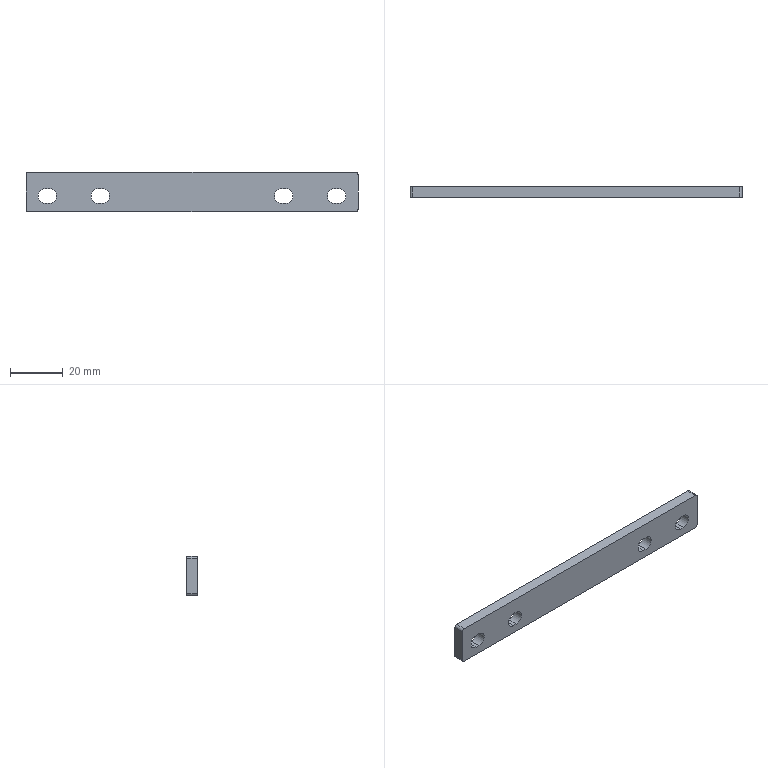Part | NX | features BREP 1 | 1 solid | 26 faces | box 125.75 x 4 x 15 mm | volume 7029 mm3 | plane 14 | cylinder 12 | commonest cylinder face diameters 5.5 x8 2 x4
STEP:
#1=CARTESIAN_POINT('',(147.026,-209.294,1985.218));
#2=VERTEX_POINT('',#1);
#3=CARTESIAN_POINT('',(147.026,-209.294,1998.218));
#4=VERTEX_POINT('',#3);
#5=CARTESIAN_POINT('',(147.026,-209.294,73.4));
#6=DIRECTION('',(0.,0.,1.));
#7=VECTOR('',#6,1000.);
#8=LINE('',#5,#7);
#9=EDGE_CURVE('',#2,#4,#8,.T.);
#10=ORIENTED_EDGE('',*,*,#9,.T.);
#11=CARTESIAN_POINT('',(146.026,-209.294,1999.218));
#12=VERTEX_POINT('',#11);
#13=CARTESIAN_POINT('',(146.026,-209.294,1998.218));
#14=DIRECTION('',(0.,1.,0.));
#15=DIRECTION('',(0.,0.,-1.));
#16=AXIS2_PLACEMENT_3D('',#13,#14,#15);
#17=CIRCLE('',#16,1.);
#18=EDGE_CURVE('',#12,#4,#17,.T.);
#19=ORIENTED_EDGE('',*,*,#18,.F.);
#20=CARTESIAN_POINT('',(22.276,-209.294,1999.218));
#21=VERTEX_POINT('',#20);
#22=CARTESIAN_POINT('',(1.713,-209.294,1999.218));
#23=DIRECTION('',(-1.,0.,0.));
#24=VECTOR('',#23,1000.);
#25=LINE('',#22,#24);
#26=EDGE_CURVE('',#12,#21,#25,.T.);
#27=ORIENTED_EDGE('',*,*,#26,.T.);
#28=CARTESIAN_POINT('',(21.276,-209.294,1998.218));
#29=VERTEX_POINT('',#28);
#30=CARTESIAN_POINT('',(22.276,-209.294,1998.218));
#31=DIRECTION('',(0.,1.,0.));
#32=DIRECTION('',(0.,0.,-1.));
#33=AXIS2_PLACEMENT_3D('',#30,#31,#32);
#34=CIRCLE('',#33,1.);
#35=EDGE_CURVE('',#29,#21,#34,.T.);
#36=ORIENTED_EDGE('',*,*,#35,.F.);
#37=CARTESIAN_POINT('',(21.276,-209.294,1985.218));
#38=VERTEX_POINT('',#37);
#39=CARTESIAN_POINT('',(21.276,-209.294,73.4));
#40=DIRECTION('',(0.,0.,-1.));
#41=VECTOR('',#40,1000.);
#42=LINE('',#39,#41);
#43=EDGE_CURVE('',#29,#38,#42,.T.);
#44=ORIENTED_EDGE('',*,*,#43,.T.);
#45=CARTESIAN_POINT('',(22.276,-209.294,1984.218));
#46=VERTEX_POINT('',#45);
#47=CARTESIAN_POINT('',(22.276,-209.294,1985.218));
#48=DIRECTION('',(0.,1.,0.));
#49=DIRECTION('',(0.,0.,1.));
#50=AXIS2_PLACEMENT_3D('',#47,#48,#49);
#51=CIRCLE('',#50,1.);
#52=EDGE_CURVE('',#46,#38,#51,.T.);
#53=ORIENTED_EDGE('',*,*,#52,.F.);
#54=CARTESIAN_POINT('',(146.026,-209.294,1984.218));
#55=VERTEX_POINT('',#54);
#56=CARTESIAN_POINT('',(1.713,-209.294,1984.218));
#57=DIRECTION('',(1.,0.,0.));
#58=VECTOR('',#57,1000.);
#59=LINE('',#56,#58);
#60=EDGE_CURVE('',#46,#55,#59,.T.);
#61=ORIENTED_EDGE('',*,*,#60,.T.);
#62=CARTESIAN_POINT('',(146.026,-209.294,1985.218));
#63=DIRECTION('',(0.,1.,0.));
#64=DIRECTION('',(0.,0.,-1.));
#65=AXIS2_PLACEMENT_3D('',#62,#63,#64);
#66=CIRCLE('',#65,1.);
#67=EDGE_CURVE('',#2,#55,#66,.T.);
#68=ORIENTED_EDGE('',*,*,#67,.F.);
#69=EDGE_LOOP('',(#10,#19,#27,#36,#44,#53,#61,#68));
#70=FACE_BOUND('',#69,.T.);
#71=CARTESIAN_POINT('',(139.651,-209.294,1992.95));
#72=VERTEX_POINT('',#71);
#73=CARTESIAN_POINT('',(139.651,-209.294,1987.45));
#74=VERTEX_POINT('',#73);
#75=CARTESIAN_POINT('',(139.651,-209.294,1990.2));
#76=DIRECTION('',(0.,1.,0.));
#77=DIRECTION('',(0.,0.,1.));
#78=AXIS2_PLACEMENT_3D('',#75,#76,#77);
#79=CIRCLE('',#78,2.75);
#80=EDGE_CURVE('',#72,#74,#79,.T.);
#81=ORIENTED_EDGE('',*,*,#80,.T.);
#82=CARTESIAN_POINT('',(138.151,-209.294,1987.45));
#83=VERTEX_POINT('',#82);
#84=CARTESIAN_POINT('',(48.651,-209.294,1987.45));
#85=DIRECTION('',(-1.,0.,0.));
#86=VECTOR('',#85,1000.);
#87=LINE('',#84,#86);
#88=EDGE_CURVE('',#74,#83,#87,.T.);
#89=ORIENTED_EDGE('',*,*,#88,.T.);
#90=CARTESIAN_POINT('',(138.151,-209.294,1992.95));
#91=VERTEX_POINT('',#90);
#92=CARTESIAN_POINT('',(138.151,-209.294,1990.2));
#93=DIRECTION('',(0.,1.,0.));
#94=DIRECTION('',(0.,0.,1.));
#95=AXIS2_PLACEMENT_3D('',#92,#93,#94);
#96=CIRCLE('',#95,2.75);
#97=EDGE_CURVE('',#83,#91,#96,.T.);
#98=ORIENTED_EDGE('',*,*,#97,.T.);
#99=CARTESIAN_POINT('',(50.151,-209.294,1992.95));
#100=DIRECTION('',(1.,0.,0.));
#101=VECTOR('',#100,1000.);
#102=LINE('',#99,#101);
#103=EDGE_CURVE('',#91,#72,#102,.T.);
#104=ORIENTED_EDGE('',*,*,#103,.T.);
#105=EDGE_LOOP('',(#81,#89,#98,#104));
#106=FACE_BOUND('',#105,.T.);
#107=CARTESIAN_POINT('',(118.151,-209.294,1992.95));
#108=VERTEX_POINT('',#107);
#109=CARTESIAN_POINT('',(119.651,-209.294,1992.95));
#110=VERTEX_POINT('',#109);
#111=CARTESIAN_POINT('',(50.151,-209.294,1992.95));
#112=DIRECTION('',(1.,0.,0.));
#113=VECTOR('',#112,1000.);
#114=LINE('',#111,#113);
#115=EDGE_CURVE('',#108,#110,#114,.T.);
#116=ORIENTED_EDGE('',*,*,#115,.T.);
#117=CARTESIAN_POINT('',(119.651,-209.294,1987.45));
#118=VERTEX_POINT('',#117);
#119=CARTESIAN_POINT('',(119.651,-209.294,1990.2));
#120=DIRECTION('',(0.,1.,0.));
#121=DIRECTION('',(0.,0.,1.));
#122=AXIS2_PLACEMENT_3D('',#119,#120,#121);
#123=CIRCLE('',#122,2.75);
#124=EDGE_CURVE('',#110,#118,#123,.T.);
#125=ORIENTED_EDGE('',*,*,#124,.T.);
#126=CARTESIAN_POINT('',(118.151,-209.294,1987.45));
#127=VERTEX_POINT('',#126);
#128=CARTESIAN_POINT('',(48.651,-209.294,1987.45));
#129=DIRECTION('',(-1.,0.,0.));
#130=VECTOR('',#129,1000.);
#131=LINE('',#128,#130);
#132=EDGE_CURVE('',#118,#127,#131,.T.);
#133=ORIENTED_EDGE('',*,*,#132,.T.);
#134=CARTESIAN_POINT('',(118.151,-209.294,1990.2));
#135=DIRECTION('',(0.,1.,0.));
#136=DIRECTION('',(0.,0.,1.));
#137=AXIS2_PLACEMENT_3D('',#134,#135,#136);
#138=CIRCLE('',#137,2.75);
#139=EDGE_CURVE('',#127,#108,#138,.T.);
#140=ORIENTED_EDGE('',*,*,#139,.T.);
#141=EDGE_LOOP('',(#116,#125,#133,#140));
#142=FACE_BOUND('',#141,.T.);
#143=CARTESIAN_POINT('',(30.151,-209.294,1992.95));
#144=VERTEX_POINT('',#143);
#145=CARTESIAN_POINT('',(30.151,-209.294,1987.45));
#146=VERTEX_POINT('',#145);
#147=CARTESIAN_POINT('',(30.151,-209.294,1990.2));
#148=DIRECTION('',(0.,1.,0.));
#149=DIRECTION('',(0.,0.,-1.));
#150=AXIS2_PLACEMENT_3D('',#147,#148,#149);
#151=CIRCLE('',#150,2.75);
#152=EDGE_CURVE('',#144,#146,#151,.T.);
#153=ORIENTED_EDGE('',*,*,#152,.T.);
#154=CARTESIAN_POINT('',(28.651,-209.294,1987.45));
#155=VERTEX_POINT('',#154);
#156=CARTESIAN_POINT('',(48.651,-209.294,1987.45));
#157=DIRECTION('',(-1.,0.,0.));
#158=VECTOR('',#157,1000.);
#159=LINE('',#156,#158);
#160=EDGE_CURVE('',#146,#155,#159,.T.);
#161=ORIENTED_EDGE('',*,*,#160,.T.);
#162=CARTESIAN_POINT('',(28.651,-209.294,1992.95));
#163=VERTEX_POINT('',#162);
#164=CARTESIAN_POINT('',(28.651,-209.294,1990.2));
#165=DIRECTION('',(0.,1.,0.));
#166=DIRECTION('',(0.,0.,-1.));
#167=AXIS2_PLACEMENT_3D('',#164,#165,#166);
#168=CIRCLE('',#167,2.75);
#169=EDGE_CURVE('',#155,#163,#168,.T.);
#170=ORIENTED_EDGE('',*,*,#169,.T.);
#171=CARTESIAN_POINT('',(50.151,-209.294,1992.95));
#172=DIRECTION('',(1.,0.,0.));
#173=VECTOR('',#172,1000.);
#174=LINE('',#171,#173);
#175=EDGE_CURVE('',#163,#144,#174,.T.);
#176=ORIENTED_EDGE('',*,*,#175,.T.);
#177=EDGE_LOOP('',(#153,#161,#170,#176));
#178=FACE_BOUND('',#177,.T.);
#179=CARTESIAN_POINT('',(50.151,-209.294,1992.95));
#180=VERTEX_POINT('',#179);
#181=CARTESIAN_POINT('',(50.151,-209.294,1987.45));
#182=VERTEX_POINT('',#181);
#183=CARTESIAN_POINT('',(50.151,-209.294,1990.2));
#184=DIRECTION('',(0.,1.,0.));
#185=DIRECTION('',(0.,0.,-1.));
#186=AXIS2_PLACEMENT_3D('',#183,#184,#185);
#187=CIRCLE('',#186,2.75);
#188=EDGE_CURVE('',#180,#182,#187,.T.);
#189=ORIENTED_EDGE('',*,*,#188,.T.);
#190=CARTESIAN_POINT('',(48.651,-209.294,1987.45));
#191=VERTEX_POINT('',#190);
#192=CARTESIAN_POINT('',(48.651,-209.294,1987.45));
#193=DIRECTION('',(-1.,0.,0.));
#194=VECTOR('',#193,1000.);
#195=LINE('',#192,#194);
#196=EDGE_CURVE('',#182,#191,#195,.T.);
#197=ORIENTED_EDGE('',*,*,#196,.T.);
#198=CARTESIAN_POINT('',(48.651,-209.294,1992.95));
#199=VERTEX_POINT('',#198);
#200=CARTESIAN_POINT('',(48.651,-209.294,1990.2));
#201=DIRECTION('',(0.,1.,0.));
#202=DIRECTION('',(0.,0.,-1.));
#203=AXIS2_PLACEMENT_3D('',#200,#201,#202);
#204=CIRCLE('',#203,2.75);
#205=EDGE_CURVE('',#191,#199,#204,.T.);
#206=ORIENTED_EDGE('',*,*,#205,.T.);
#207=CARTESIAN_POINT('',(50.151,-209.294,1992.95));
#208=DIRECTION('',(1.,0.,0.));
#209=VECTOR('',#208,1000.);
#210=LINE('',#207,#209);
#211=EDGE_CURVE('',#199,#180,#210,.T.);
#212=ORIENTED_EDGE('',*,*,#211,.T.);
#213=EDGE_LOOP('',(#189,#197,#206,#212));
#214=FACE_BOUND('',#213,.T.);
#215=CARTESIAN_POINT('',(1.713,-209.294,73.4));
#216=DIRECTION('',(0.,-1.,0.));
#217=DIRECTION('',(0.,0.,1.));
#218=AXIS2_PLACEMENT_3D('',#215,#216,#217);
#219=PLANE('',#218);
#220=ADVANCED_FACE('',(#70,#106,#142,#178,#214),#219,.T.);
#221=CARTESIAN_POINT('',(147.026,-205.294,1985.218));
#222=VERTEX_POINT('',#221);
#223=CARTESIAN_POINT('',(147.026,-206.294,1985.218));
#224=DIRECTION('',(0.,-1.,0.));
#225=VECTOR('',#224,1000.);
#226=LINE('',#223,#225);
#227=EDGE_CURVE('',#222,#2,#226,.T.);
#228=ORIENTED_EDGE('',*,*,#227,.F.);
#229=CARTESIAN_POINT('',(147.026,-205.294,1998.218));
#230=VERTEX_POINT('',#229);
#231=CARTESIAN_POINT('',(147.026,-205.294,2020.218));
#232=DIRECTION('',(0.,0.,-1.));
#233=VECTOR('',#232,1000.);
#234=LINE('',#231,#233);
#235=EDGE_CURVE('',#230,#222,#234,.T.);
#236=ORIENTED_EDGE('',*,*,#235,.F.);
#237=CARTESIAN_POINT('',(147.026,-206.294,1998.218));
#238=DIRECTION('',(0.,1.,0.));
#239=VECTOR('',#238,1000.);
#240=LINE('',#237,#239);
#241=EDGE_CURVE('',#4,#230,#240,.T.);
#242=ORIENTED_EDGE('',*,*,#241,.F.);
#243=ORIENTED_EDGE('',*,*,#9,.F.);
#244=EDGE_LOOP('',(#228,#236,#242,#243));
#245=FACE_BOUND('',#244,.T.);
#246=CARTESIAN_POINT('',(147.026,-206.294,2020.218));
#247=DIRECTION('',(-1.,0.,0.));
#248=DIRECTION('',(0.,0.,-1.));
#249=AXIS2_PLACEMENT_3D('',#246,#247,#248);
#250=PLANE('',#249);
#251=ADVANCED_FACE('',(#245),#250,.F.);
#252=CARTESIAN_POINT('',(22.276,-205.294,1984.218));
#253=VERTEX_POINT('',#252);
#254=CARTESIAN_POINT('',(22.276,-206.294,1984.218));
#255=DIRECTION('',(0.,1.,0.));
#256=VECTOR('',#255,1000.);
#257=LINE('',#254,#256);
#258=EDGE_CURVE('',#46,#253,#257,.T.);
#259=ORIENTED_EDGE('',*,*,#258,.T.);
#260=CARTESIAN_POINT('',(146.026,-205.294,1984.218));
#261=VERTEX_POINT('',#260);
#262=CARTESIAN_POINT('',(21.276,-205.294,1984.218));
#263=DIRECTION('',(1.,0.,0.));
#264=VECTOR('',#263,1000.);
#265=LINE('',#262,#264);
#266=EDGE_CURVE('',#253,#261,#265,.T.);
#267=ORIENTED_EDGE('',*,*,#266,.T.);
#268=CARTESIAN_POINT('',(146.026,-206.294,1984.218));
#269=DIRECTION('',(0.,-1.,0.));
#270=VECTOR('',#269,1000.);
#271=LINE('',#268,#270);
#272=EDGE_CURVE('',#261,#55,#271,.T.);
#273=ORIENTED_EDGE('',*,*,#272,.T.);
#274=ORIENTED_EDGE('',*,*,#60,.F.);
#275=EDGE_LOOP('',(#259,#267,#273,#274));
#276=FACE_BOUND('',#275,.T.);
#277=CARTESIAN_POINT('',(21.276,-206.294,1984.218));
#278=DIRECTION('',(0.,0.,-1.));
#279=DIRECTION('',(1.,0.,0.));
#280=AXIS2_PLACEMENT_3D('',#277,#278,#279);
#281=PLANE('',#280);
#282=ADVANCED_FACE('',(#276),#281,.T.);
#283=CARTESIAN_POINT('',(21.276,-205.294,1998.218));
#284=VERTEX_POINT('',#283);
#285=CARTESIAN_POINT('',(21.276,-205.294,1985.218));
#286=VERTEX_POINT('',#285);
#287=CARTESIAN_POINT('',(21.276,-205.294,2020.218));
#288=DIRECTION('',(0.,0.,-1.));
#289=VECTOR('',#288,1000.);
#290=LINE('',#287,#289);
#291=EDGE_CURVE('',#284,#286,#290,.T.);
#292=ORIENTED_EDGE('',*,*,#291,.T.);
#293=CARTESIAN_POINT('',(21.276,-206.294,1985.218));
#294=DIRECTION('',(0.,-1.,0.));
#295=VECTOR('',#294,1000.);
#296=LINE('',#293,#295);
#297=EDGE_CURVE('',#286,#38,#296,.T.);
#298=ORIENTED_EDGE('',*,*,#297,.T.);
#299=ORIENTED_EDGE('',*,*,#43,.F.);
#300=CARTESIAN_POINT('',(21.276,-206.294,1998.218));
#301=DIRECTION('',(0.,1.,0.));
#302=VECTOR('',#301,1000.);
#303=LINE('',#300,#302);
#304=EDGE_CURVE('',#29,#284,#303,.T.);
#305=ORIENTED_EDGE('',*,*,#304,.T.);
#306=EDGE_LOOP('',(#292,#298,#299,#305));
#307=FACE_BOUND('',#306,.T.);
#308=CARTESIAN_POINT('',(21.276,-206.294,2020.218));
#309=DIRECTION('',(-1.,0.,0.));
#310=DIRECTION('',(0.,0.,-1.));
#311=AXIS2_PLACEMENT_3D('',#308,#309,#310);
#312=PLANE('',#311);
#313=ADVANCED_FACE('',(#307),#312,.T.);
#314=ORIENTED_EDGE('',*,*,#26,.F.);
#315=CARTESIAN_POINT('',(146.026,-205.294,1999.218));
#316=VERTEX_POINT('',#315);
#317=CARTESIAN_POINT('',(146.026,-206.294,1999.218));
#318=DIRECTION('',(0.,1.,0.));
#319=VECTOR('',#318,1000.);
#320=LINE('',#317,#319);
#321=EDGE_CURVE('',#12,#316,#320,.T.);
#322=ORIENTED_EDGE('',*,*,#321,.T.);
#323=CARTESIAN_POINT('',(22.276,-205.294,1999.218));
#324=VERTEX_POINT('',#323);
#325=CARTESIAN_POINT('',(151.826,-205.294,1999.218));
#326=DIRECTION('',(-1.,0.,0.));
#327=VECTOR('',#326,1000.);
#328=LINE('',#325,#327);
#329=EDGE_CURVE('',#316,#324,#328,.T.);
#330=ORIENTED_EDGE('',*,*,#329,.T.);
#331=CARTESIAN_POINT('',(22.276,-206.294,1999.218));
#332=DIRECTION('',(0.,-1.,0.));
#333=VECTOR('',#332,1000.);
#334=LINE('',#331,#333);
#335=EDGE_CURVE('',#324,#21,#334,.T.);
#336=ORIENTED_EDGE('',*,*,#335,.T.);
#337=EDGE_LOOP('',(#314,#322,#330,#336));
#338=FACE_BOUND('',#337,.T.);
#339=CARTESIAN_POINT('',(151.826,-206.294,1999.218));
#340=DIRECTION('',(0.,0.,1.));
#341=DIRECTION('',(-1.,0.,0.));
#342=AXIS2_PLACEMENT_3D('',#339,#340,#341);
#343=PLANE('',#342);
#344=ADVANCED_FACE('',(#338),#343,.T.);
#345=ORIENTED_EDGE('',*,*,#80,.F.);
#346=CARTESIAN_POINT('',(139.651,-205.294,1992.95));
#347=VERTEX_POINT('',#346);
#348=CARTESIAN_POINT('',(139.651,-206.294,1992.95));
#349=DIRECTION('',(0.,-1.,0.));
#350=VECTOR('',#349,1000.);
#351=LINE('',#348,#350);
#352=EDGE_CURVE('',#347,#72,#351,.T.);
#353=ORIENTED_EDGE('',*,*,#352,.F.);
#354=CARTESIAN_POINT('',(139.651,-205.294,1987.45));
#355=VERTEX_POINT('',#354);
#356=CARTESIAN_POINT('',(139.651,-205.294,1990.2));
#357=DIRECTION('',(0.,-1.,0.));
#358=DIRECTION('',(0.,0.,1.));
#359=AXIS2_PLACEMENT_3D('',#356,#357,#358);
#360=CIRCLE('',#359,2.75);
#361=EDGE_CURVE('',#355,#347,#360,.T.);
#362=ORIENTED_EDGE('',*,*,#361,.F.);
#363=CARTESIAN_POINT('',(139.651,-206.294,1987.45));
#364=DIRECTION('',(0.,1.,0.));
#365=VECTOR('',#364,1000.);
#366=LINE('',#363,#365);
#367=EDGE_CURVE('',#74,#355,#366,.T.);
#368=ORIENTED_EDGE('',*,*,#367,.F.);
#369=EDGE_LOOP('',(#345,#353,#362,#368));
#370=FACE_BOUND('',#369,.T.);
#371=CARTESIAN_POINT('',(139.651,-206.294,1990.2));
#372=DIRECTION('',(0.,1.,0.));
#373=DIRECTION('',(0.,0.,-1.));
#374=AXIS2_PLACEMENT_3D('',#371,#372,#373);
#375=CYLINDRICAL_SURFACE('',#374,2.75);
#376=ADVANCED_FACE('',(#370),#375,.F.);
#377=ORIENTED_EDGE('',*,*,#97,.F.);
#378=CARTESIAN_POINT('',(138.151,-205.294,1987.45));
#379=VERTEX_POINT('',#378);
#380=CARTESIAN_POINT('',(138.151,-206.294,1987.45));
#381=DIRECTION('',(0.,-1.,0.));
#382=VECTOR('',#381,1000.);
#383=LINE('',#380,#382);
#384=EDGE_CURVE('',#379,#83,#383,.T.);
#385=ORIENTED_EDGE('',*,*,#384,.F.);
#386=CARTESIAN_POINT('',(138.151,-205.294,1992.95));
#387=VERTEX_POINT('',#386);
#388=CARTESIAN_POINT('',(138.151,-205.294,1990.2));
#389=DIRECTION('',(0.,-1.,0.));
#390=DIRECTION('',(0.,0.,1.));
#391=AXIS2_PLACEMENT_3D('',#388,#389,#390);
#392=CIRCLE('',#391,2.75);
#393=EDGE_CURVE('',#387,#379,#392,.T.);
#394=ORIENTED_EDGE('',*,*,#393,.F.);
#395=CARTESIAN_POINT('',(138.151,-206.294,1992.95));
#396=DIRECTION('',(0.,1.,0.));
#397=VECTOR('',#396,1000.);
#398=LINE('',#395,#397);
#399=EDGE_CURVE('',#91,#387,#398,.T.);
#400=ORIENTED_EDGE('',*,*,#399,.F.);
#401=EDGE_LOOP('',(#377,#385,#394,#400));
#402=FACE_BOUND('',#401,.T.);
#403=CARTESIAN_POINT('',(138.151,-206.294,1990.2));
#404=DIRECTION('',(0.,1.,0.));
#405=DIRECTION('',(0.,0.,-1.));
#406=AXIS2_PLACEMENT_3D('',#403,#404,#405);
#407=CYLINDRICAL_SURFACE('',#406,2.75);
#408=ADVANCED_FACE('',(#402),#407,.F.);
#409=ORIENTED_EDGE('',*,*,#124,.F.);
#410=CARTESIAN_POINT('',(119.651,-205.294,1992.95));
#411=VERTEX_POINT('',#410);
#412=CARTESIAN_POINT('',(119.651,-206.294,1992.95));
#413=DIRECTION('',(0.,-1.,0.));
#414=VECTOR('',#413,1000.);
#415=LINE('',#412,#414);
#416=EDGE_CURVE('',#411,#110,#415,.T.);
#417=ORIENTED_EDGE('',*,*,#416,.F.);
#418=CARTESIAN_POINT('',(119.651,-205.294,1987.45));
#419=VERTEX_POINT('',#418);
#420=CARTESIAN_POINT('',(119.651,-205.294,1990.2));
#421=DIRECTION('',(0.,-1.,0.));
#422=DIRECTION('',(0.,0.,1.));
#423=AXIS2_PLACEMENT_3D('',#420,#421,#422);
#424=CIRCLE('',#423,2.75);
#425=EDGE_CURVE('',#419,#411,#424,.T.);
#426=ORIENTED_EDGE('',*,*,#425,.F.);
#427=CARTESIAN_POINT('',(119.651,-206.294,1987.45));
#428=DIRECTION('',(0.,1.,0.));
#429=VECTOR('',#428,1000.);
#430=LINE('',#427,#429);
#431=EDGE_CURVE('',#118,#419,#430,.T.);
#432=ORIENTED_EDGE('',*,*,#431,.F.);
#433=EDGE_LOOP('',(#409,#417,#426,#432));
#434=FACE_BOUND('',#433,.T.);
#435=CARTESIAN_POINT('',(119.651,-206.294,1990.2));
#436=DIRECTION('',(0.,1.,0.));
#437=DIRECTION('',(0.,0.,-1.));
#438=AXIS2_PLACEMENT_3D('',#435,#436,#437);
#439=CYLINDRICAL_SURFACE('',#438,2.75);
#440=ADVANCED_FACE('',(#434),#439,.F.);
#441=CARTESIAN_POINT('',(118.151,-205.294,1992.95));
#442=VERTEX_POINT('',#441);
#443=CARTESIAN_POINT('',(118.151,-205.294,1987.45));
#444=VERTEX_POINT('',#443);
#445=CARTESIAN_POINT('',(118.151,-205.294,1990.2));
#446=DIRECTION('',(0.,-1.,0.));
#447=DIRECTION('',(0.,0.,1.));
#448=AXIS2_PLACEMENT_3D('',#445,#446,#447);
#449=CIRCLE('',#448,2.75);
#450=EDGE_CURVE('',#442,#444,#449,.T.);
#451=ORIENTED_EDGE('',*,*,#450,.F.);
#452=CARTESIAN_POINT('',(118.151,-206.294,1992.95));
#453=DIRECTION('',(0.,1.,0.));
#454=VECTOR('',#453,1000.);
#455=LINE('',#452,#454);
#456=EDGE_CURVE('',#108,#442,#455,.T.);
#457=ORIENTED_EDGE('',*,*,#456,.F.);
#458=ORIENTED_EDGE('',*,*,#139,.F.);
#459=CARTESIAN_POINT('',(118.151,-206.294,1987.45));
#460=DIRECTION('',(0.,-1.,0.));
#461=VECTOR('',#460,1000.);
#462=LINE('',#459,#461);
#463=EDGE_CURVE('',#444,#127,#462,.T.);
#464=ORIENTED_EDGE('',*,*,#463,.F.);
#465=EDGE_LOOP('',(#451,#457,#458,#464));
#466=FACE_BOUND('',#465,.T.);
#467=CARTESIAN_POINT('',(118.151,-206.294,1990.2));
#468=DIRECTION('',(0.,1.,0.));
#469=DIRECTION('',(0.,0.,-1.));
#470=AXIS2_PLACEMENT_3D('',#467,#468,#469);
#471=CYLINDRICAL_SURFACE('',#470,2.75);
#472=ADVANCED_FACE('',(#466),#471,.F.);
#473=ORIENTED_EDGE('',*,*,#152,.F.);
#474=CARTESIAN_POINT('',(30.151,-205.294,1992.95));
#475=VERTEX_POINT('',#474);
#476=CARTESIAN_POINT('',(30.151,-206.294,1992.95));
#477=DIRECTION('',(0.,-1.,0.));
#478=VECTOR('',#477,1000.);
#479=LINE('',#476,#478);
#480=EDGE_CURVE('',#475,#144,#479,.T.);
#481=ORIENTED_EDGE('',*,*,#480,.F.);
#482=CARTESIAN_POINT('',(30.151,-205.294,1987.45));
#483=VERTEX_POINT('',#482);
#484=CARTESIAN_POINT('',(30.151,-205.294,1990.2));
#485=DIRECTION('',(0.,-1.,0.));
#486=DIRECTION('',(0.,0.,-1.));
#487=AXIS2_PLACEMENT_3D('',#484,#485,#486);
#488=CIRCLE('',#487,2.75);
#489=EDGE_CURVE('',#483,#475,#488,.T.);
#490=ORIENTED_EDGE('',*,*,#489,.F.);
#491=CARTESIAN_POINT('',(30.151,-206.294,1987.45));
#492=DIRECTION('',(0.,1.,0.));
#493=VECTOR('',#492,1000.);
#494=LINE('',#491,#493);
#495=EDGE_CURVE('',#146,#483,#494,.T.);
#496=ORIENTED_EDGE('',*,*,#495,.F.);
#497=EDGE_LOOP('',(#473,#481,#490,#496));
#498=FACE_BOUND('',#497,.T.);
#499=CARTESIAN_POINT('',(30.151,-206.294,1990.2));
#500=DIRECTION('',(0.,-1.,0.));
#501=DIRECTION('',(0.,0.,1.));
#502=AXIS2_PLACEMENT_3D('',#499,#500,#501);
#503=CYLINDRICAL_SURFACE('',#502,2.75);
#504=ADVANCED_FACE('',(#498),#503,.F.);
#505=ORIENTED_EDGE('',*,*,#169,.F.);
#506=CARTESIAN_POINT('',(28.651,-205.294,1987.45));
#507=VERTEX_POINT('',#506);
#508=CARTESIAN_POINT('',(28.651,-206.294,1987.45));
#509=DIRECTION('',(0.,-1.,0.));
#510=VECTOR('',#509,1000.);
#511=LINE('',#508,#510);
#512=EDGE_CURVE('',#507,#155,#511,.T.);
#513=ORIENTED_EDGE('',*,*,#512,.F.);
#514=CARTESIAN_POINT('',(28.651,-205.294,1992.95));
#515=VERTEX_POINT('',#514);
#516=CARTESIAN_POINT('',(28.651,-205.294,1990.2));
#517=DIRECTION('',(0.,-1.,0.));
#518=DIRECTION('',(0.,0.,-1.));
#519=AXIS2_PLACEMENT_3D('',#516,#517,#518);
#520=CIRCLE('',#519,2.75);
#521=EDGE_CURVE('',#515,#507,#520,.T.);
#522=ORIENTED_EDGE('',*,*,#521,.F.);
#523=CARTESIAN_POINT('',(28.651,-206.294,1992.95));
#524=DIRECTION('',(0.,1.,0.));
#525=VECTOR('',#524,1000.);
#526=LINE('',#523,#525);
#527=EDGE_CURVE('',#163,#515,#526,.T.);
#528=ORIENTED_EDGE('',*,*,#527,.F.);
#529=EDGE_LOOP('',(#505,#513,#522,#528));
#530=FACE_BOUND('',#529,.T.);
#531=CARTESIAN_POINT('',(28.651,-206.294,1990.2));
#532=DIRECTION('',(0.,-1.,0.));
#533=DIRECTION('',(0.,0.,1.));
#534=AXIS2_PLACEMENT_3D('',#531,#532,#533);
#535=CYLINDRICAL_SURFACE('',#534,2.75);
#536=ADVANCED_FACE('',(#530),#535,.F.);
#537=ORIENTED_EDGE('',*,*,#188,.F.);
#538=CARTESIAN_POINT('',(50.151,-205.294,1992.95));
#539=VERTEX_POINT('',#538);
#540=CARTESIAN_POINT('',(50.151,-206.294,1992.95));
#541=DIRECTION('',(0.,-1.,0.));
#542=VECTOR('',#541,1000.);
#543=LINE('',#540,#542);
#544=EDGE_CURVE('',#539,#180,#543,.T.);
#545=ORIENTED_EDGE('',*,*,#544,.F.);
#546=CARTESIAN_POINT('',(50.151,-205.294,1987.45));
#547=VERTEX_POINT('',#546);
#548=CARTESIAN_POINT('',(50.151,-205.294,1990.2));
#549=DIRECTION('',(0.,-1.,0.));
#550=DIRECTION('',(0.,0.,-1.));
#551=AXIS2_PLACEMENT_3D('',#548,#549,#550);
#552=CIRCLE('',#551,2.75);
#553=EDGE_CURVE('',#547,#539,#552,.T.);
#554=ORIENTED_EDGE('',*,*,#553,.F.);
#555=CARTESIAN_POINT('',(50.151,-206.294,1987.45));
#556=DIRECTION('',(0.,1.,0.));
#557=VECTOR('',#556,1000.);
#558=LINE('',#555,#557);
#559=EDGE_CURVE('',#182,#547,#558,.T.);
#560=ORIENTED_EDGE('',*,*,#559,.F.);
#561=EDGE_LOOP('',(#537,#545,#554,#560));
#562=FACE_BOUND('',#561,.T.);
#563=CARTESIAN_POINT('',(50.151,-206.294,1990.2));
#564=DIRECTION('',(0.,-1.,0.));
#565=DIRECTION('',(0.,0.,1.));
#566=AXIS2_PLACEMENT_3D('',#563,#564,#565);
#567=CYLINDRICAL_SURFACE('',#566,2.75);
#568=ADVANCED_FACE('',(#562),#567,.F.);
#569=ORIENTED_EDGE('',*,*,#205,.F.);
#570=CARTESIAN_POINT('',(48.651,-205.294,1987.45));
#571=VERTEX_POINT('',#570);
#572=CARTESIAN_POINT('',(48.651,-206.294,1987.45));
#573=DIRECTION('',(0.,-1.,0.));
#574=VECTOR('',#573,1000.);
#575=LINE('',#572,#574);
#576=EDGE_CURVE('',#571,#191,#575,.T.);
#577=ORIENTED_EDGE('',*,*,#576,.F.);
#578=CARTESIAN_POINT('',(48.651,-205.294,1992.95));
#579=VERTEX_POINT('',#578);
#580=CARTESIAN_POINT('',(48.651,-205.294,1990.2));
#581=DIRECTION('',(0.,-1.,0.));
#582=DIRECTION('',(0.,0.,-1.));
#583=AXIS2_PLACEMENT_3D('',#580,#581,#582);
#584=CIRCLE('',#583,2.75);
#585=EDGE_CURVE('',#579,#571,#584,.T.);
#586=ORIENTED_EDGE('',*,*,#585,.F.);
#587=CARTESIAN_POINT('',(48.651,-206.294,1992.95));
#588=DIRECTION('',(0.,1.,0.));
#589=VECTOR('',#588,1000.);
#590=LINE('',#587,#589);
#591=EDGE_CURVE('',#199,#579,#590,.T.);
#592=ORIENTED_EDGE('',*,*,#591,.F.);
#593=EDGE_LOOP('',(#569,#577,#586,#592));
#594=FACE_BOUND('',#593,.T.);
#595=CARTESIAN_POINT('',(48.651,-206.294,1990.2));
#596=DIRECTION('',(0.,-1.,0.));
#597=DIRECTION('',(0.,0.,1.));
#598=AXIS2_PLACEMENT_3D('',#595,#596,#597);
#599=CYLINDRICAL_SURFACE('',#598,2.75);
#600=ADVANCED_FACE('',(#594),#599,.F.);
#601=ORIENTED_EDGE('',*,*,#227,.T.);
#602=ORIENTED_EDGE('',*,*,#67,.T.);
#603=ORIENTED_EDGE('',*,*,#272,.F.);
#604=CARTESIAN_POINT('',(146.026,-205.294,1985.218));
#605=DIRECTION('',(0.,-1.,0.));
#606=DIRECTION('',(0.,0.,-1.));
#607=AXIS2_PLACEMENT_3D('',#604,#605,#606);
#608=CIRCLE('',#607,1.);
#609=EDGE_CURVE('',#261,#222,#608,.T.);
#610=ORIENTED_EDGE('',*,*,#609,.T.);
#611=EDGE_LOOP('',(#601,#602,#603,#610));
#612=FACE_BOUND('',#611,.T.);
#613=CARTESIAN_POINT('',(146.026,-213.205,1985.218));
#614=DIRECTION('',(0.,-1.,0.));
#615=DIRECTION('',(0.,0.,1.));
#616=AXIS2_PLACEMENT_3D('',#613,#614,#615);
#617=CYLINDRICAL_SURFACE('',#616,1.);
#618=ADVANCED_FACE('',(#612),#617,.T.);
#619=CARTESIAN_POINT('',(146.026,-205.294,1998.218));
#620=DIRECTION('',(0.,-1.,0.));
#621=DIRECTION('',(0.,0.,-1.));
#622=AXIS2_PLACEMENT_3D('',#619,#620,#621);
#623=CIRCLE('',#622,1.);
#624=EDGE_CURVE('',#230,#316,#623,.T.);
#625=ORIENTED_EDGE('',*,*,#624,.F.);
#626=ORIENTED_EDGE('',*,*,#235,.T.);
#627=ORIENTED_EDGE('',*,*,#609,.F.);
#628=ORIENTED_EDGE('',*,*,#266,.F.);
#629=CARTESIAN_POINT('',(22.276,-205.294,1985.218));
#630=DIRECTION('',(0.,-1.,0.));
#631=DIRECTION('',(0.,0.,1.));
#632=AXIS2_PLACEMENT_3D('',#629,#630,#631);
#633=CIRCLE('',#632,1.);
#634=EDGE_CURVE('',#286,#253,#633,.T.);
#635=ORIENTED_EDGE('',*,*,#634,.F.);
#636=ORIENTED_EDGE('',*,*,#291,.F.);
#637=CARTESIAN_POINT('',(22.276,-205.294,1998.218));
#638=DIRECTION('',(0.,-1.,0.));
#639=DIRECTION('',(0.,0.,-1.));
#640=AXIS2_PLACEMENT_3D('',#637,#638,#639);
#641=CIRCLE('',#640,1.);
#642=EDGE_CURVE('',#324,#284,#641,.T.);
#643=ORIENTED_EDGE('',*,*,#642,.F.);
#644=ORIENTED_EDGE('',*,*,#329,.F.);
#645=EDGE_LOOP('',(#625,#626,#627,#628,#635,#636,#643,#644));
#646=FACE_BOUND('',#645,.T.);
#647=ORIENTED_EDGE('',*,*,#553,.T.);
#648=CARTESIAN_POINT('',(1.713,-205.294,1992.95));
#649=DIRECTION('',(1.,0.,0.));
#650=VECTOR('',#649,1000.);
#651=LINE('',#648,#650);
#652=EDGE_CURVE('',#579,#539,#651,.T.);
#653=ORIENTED_EDGE('',*,*,#652,.F.);
#654=ORIENTED_EDGE('',*,*,#585,.T.);
#655=CARTESIAN_POINT('',(1.713,-205.294,1987.45));
#656=DIRECTION('',(-1.,0.,0.));
#657=VECTOR('',#656,1000.);
#658=LINE('',#655,#657);
#659=EDGE_CURVE('',#547,#571,#658,.T.);
#660=ORIENTED_EDGE('',*,*,#659,.F.);
#661=EDGE_LOOP('',(#647,#653,#654,#660));
#662=FACE_BOUND('',#661,.T.);
#663=ORIENTED_EDGE('',*,*,#521,.T.);
#664=CARTESIAN_POINT('',(1.713,-205.294,1987.45));
#665=DIRECTION('',(-1.,0.,0.));
#666=VECTOR('',#665,1000.);
#667=LINE('',#664,#666);
#668=EDGE_CURVE('',#483,#507,#667,.T.);
#669=ORIENTED_EDGE('',*,*,#668,.F.);
#670=ORIENTED_EDGE('',*,*,#489,.T.);
#671=CARTESIAN_POINT('',(1.713,-205.294,1992.95));
#672=DIRECTION('',(1.,0.,0.));
#673=VECTOR('',#672,1000.);
#674=LINE('',#671,#673);
#675=EDGE_CURVE('',#515,#475,#674,.T.);
#676=ORIENTED_EDGE('',*,*,#675,.F.);
#677=EDGE_LOOP('',(#663,#669,#670,#676));
#678=FACE_BOUND('',#677,.T.);
#679=ORIENTED_EDGE('',*,*,#450,.T.);
#680=CARTESIAN_POINT('',(1.713,-205.294,1987.45));
#681=DIRECTION('',(-1.,0.,0.));
#682=VECTOR('',#681,1000.);
#683=LINE('',#680,#682);
#684=EDGE_CURVE('',#419,#444,#683,.T.);
#685=ORIENTED_EDGE('',*,*,#684,.F.);
#686=ORIENTED_EDGE('',*,*,#425,.T.);
#687=CARTESIAN_POINT('',(1.713,-205.294,1992.95));
#688=DIRECTION('',(1.,0.,0.));
#689=VECTOR('',#688,1000.);
#690=LINE('',#687,#689);
#691=EDGE_CURVE('',#442,#411,#690,.T.);
#692=ORIENTED_EDGE('',*,*,#691,.F.);
#693=EDGE_LOOP('',(#679,#685,#686,#692));
#694=FACE_BOUND('',#693,.T.);
#695=CARTESIAN_POINT('',(1.713,-205.294,1987.45));
#696=DIRECTION('',(-1.,0.,0.));
#697=VECTOR('',#696,1000.);
#698=LINE('',#695,#697);
#699=EDGE_CURVE('',#355,#379,#698,.T.);
#700=ORIENTED_EDGE('',*,*,#699,.F.);
#701=ORIENTED_EDGE('',*,*,#361,.T.);
#702=CARTESIAN_POINT('',(1.713,-205.294,1992.95));
#703=DIRECTION('',(1.,0.,0.));
#704=VECTOR('',#703,1000.);
#705=LINE('',#702,#704);
#706=EDGE_CURVE('',#387,#347,#705,.T.);
#707=ORIENTED_EDGE('',*,*,#706,.F.);
#708=ORIENTED_EDGE('',*,*,#393,.T.);
#709=EDGE_LOOP('',(#700,#701,#707,#708));
#710=FACE_BOUND('',#709,.T.);
#711=CARTESIAN_POINT('',(1.713,-205.294,73.4));
#712=DIRECTION('',(0.,-1.,0.));
#713=DIRECTION('',(0.,0.,1.));
#714=AXIS2_PLACEMENT_3D('',#711,#712,#713);
#715=PLANE('',#714);
#716=ADVANCED_FACE('',(#646,#662,#678,#694,#710),#715,.F.);
#717=ORIENTED_EDGE('',*,*,#18,.T.);
#718=ORIENTED_EDGE('',*,*,#241,.T.);
#719=ORIENTED_EDGE('',*,*,#624,.T.);
#720=ORIENTED_EDGE('',*,*,#321,.F.);
#721=EDGE_LOOP('',(#717,#718,#719,#720));
#722=FACE_BOUND('',#721,.T.);
#723=CARTESIAN_POINT('',(146.026,-207.294,1998.218));
#724=DIRECTION('',(0.,-1.,0.));
#725=DIRECTION('',(0.,0.,1.));
#726=AXIS2_PLACEMENT_3D('',#723,#724,#725);
#727=CYLINDRICAL_SURFACE('',#726,1.);
#728=ADVANCED_FACE('',(#722),#727,.T.);
#729=ORIENTED_EDGE('',*,*,#297,.F.);
#730=ORIENTED_EDGE('',*,*,#634,.T.);
#731=ORIENTED_EDGE('',*,*,#258,.F.);
#732=ORIENTED_EDGE('',*,*,#52,.T.);
#733=EDGE_LOOP('',(#729,#730,#731,#732));
#734=FACE_BOUND('',#733,.T.);
#735=CARTESIAN_POINT('',(22.276,-213.205,1985.218));
#736=DIRECTION('',(0.,1.,0.));
#737=DIRECTION('',(0.,0.,-1.));
#738=AXIS2_PLACEMENT_3D('',#735,#736,#737);
#739=CYLINDRICAL_SURFACE('',#738,1.);
#740=ADVANCED_FACE('',(#734),#739,.T.);
#741=ORIENTED_EDGE('',*,*,#35,.T.);
#742=ORIENTED_EDGE('',*,*,#335,.F.);
#743=ORIENTED_EDGE('',*,*,#642,.T.);
#744=ORIENTED_EDGE('',*,*,#304,.F.);
#745=EDGE_LOOP('',(#741,#742,#743,#744));
#746=FACE_BOUND('',#745,.T.);
#747=CARTESIAN_POINT('',(22.276,-207.294,1998.218));
#748=DIRECTION('',(0.,-1.,0.));
#749=DIRECTION('',(0.,0.,1.));
#750=AXIS2_PLACEMENT_3D('',#747,#748,#749);
#751=CYLINDRICAL_SURFACE('',#750,1.);
#752=ADVANCED_FACE('',(#746),#751,.T.);
#753=ORIENTED_EDGE('',*,*,#88,.F.);
#754=ORIENTED_EDGE('',*,*,#367,.T.);
#755=ORIENTED_EDGE('',*,*,#699,.T.);
#756=ORIENTED_EDGE('',*,*,#384,.T.);
#757=EDGE_LOOP('',(#753,#754,#755,#756));
#758=FACE_BOUND('',#757,.T.);
#759=CARTESIAN_POINT('',(48.651,-206.294,1987.45));
#760=DIRECTION('',(0.,0.,-1.));
#761=DIRECTION('',(1.,0.,0.));
#762=AXIS2_PLACEMENT_3D('',#759,#760,#761);
#763=PLANE('',#762);
#764=ADVANCED_FACE('',(#758),#763,.F.);
#765=ORIENTED_EDGE('',*,*,#352,.T.);
#766=ORIENTED_EDGE('',*,*,#103,.F.);
#767=ORIENTED_EDGE('',*,*,#399,.T.);
#768=ORIENTED_EDGE('',*,*,#706,.T.);
#769=EDGE_LOOP('',(#765,#766,#767,#768));
#770=FACE_BOUND('',#769,.T.);
#771=CARTESIAN_POINT('',(50.151,-206.294,1992.95));
#772=DIRECTION('',(0.,0.,1.));
#773=DIRECTION('',(-1.,0.,0.));
#774=AXIS2_PLACEMENT_3D('',#771,#772,#773);
#775=PLANE('',#774);
#776=ADVANCED_FACE('',(#770),#775,.F.);
#777=ORIENTED_EDGE('',*,*,#132,.F.);
#778=ORIENTED_EDGE('',*,*,#431,.T.);
#779=ORIENTED_EDGE('',*,*,#684,.T.);
#780=ORIENTED_EDGE('',*,*,#463,.T.);
#781=EDGE_LOOP('',(#777,#778,#779,#780));
#782=FACE_BOUND('',#781,.T.);
#783=CARTESIAN_POINT('',(48.651,-206.294,1987.45));
#784=DIRECTION('',(0.,0.,-1.));
#785=DIRECTION('',(1.,0.,0.));
#786=AXIS2_PLACEMENT_3D('',#783,#784,#785);
#787=PLANE('',#786);
#788=ADVANCED_FACE('',(#782),#787,.F.);
#789=ORIENTED_EDGE('',*,*,#416,.T.);
#790=ORIENTED_EDGE('',*,*,#115,.F.);
#791=ORIENTED_EDGE('',*,*,#456,.T.);
#792=ORIENTED_EDGE('',*,*,#691,.T.);
#793=EDGE_LOOP('',(#789,#790,#791,#792));
#794=FACE_BOUND('',#793,.T.);
#795=CARTESIAN_POINT('',(50.151,-206.294,1992.95));
#796=DIRECTION('',(0.,0.,1.));
#797=DIRECTION('',(-1.,0.,0.));
#798=AXIS2_PLACEMENT_3D('',#795,#796,#797);
#799=PLANE('',#798);
#800=ADVANCED_FACE('',(#794),#799,.F.);
#801=ORIENTED_EDGE('',*,*,#495,.T.);
#802=ORIENTED_EDGE('',*,*,#668,.T.);
#803=ORIENTED_EDGE('',*,*,#512,.T.);
#804=ORIENTED_EDGE('',*,*,#160,.F.);
#805=EDGE_LOOP('',(#801,#802,#803,#804));
#806=FACE_BOUND('',#805,.T.);
#807=CARTESIAN_POINT('',(48.651,-206.294,1987.45));
#808=DIRECTION('',(0.,0.,-1.));
#809=DIRECTION('',(1.,0.,0.));
#810=AXIS2_PLACEMENT_3D('',#807,#808,#809);
#811=PLANE('',#810);
#812=ADVANCED_FACE('',(#806),#811,.F.);
#813=ORIENTED_EDGE('',*,*,#527,.T.);
#814=ORIENTED_EDGE('',*,*,#675,.T.);
#815=ORIENTED_EDGE('',*,*,#480,.T.);
#816=ORIENTED_EDGE('',*,*,#175,.F.);
#817=EDGE_LOOP('',(#813,#814,#815,#816));
#818=FACE_BOUND('',#817,.T.);
#819=CARTESIAN_POINT('',(50.151,-206.294,1992.95));
#820=DIRECTION('',(0.,0.,1.));
#821=DIRECTION('',(-1.,0.,0.));
#822=AXIS2_PLACEMENT_3D('',#819,#820,#821);
#823=PLANE('',#822);
#824=ADVANCED_FACE('',(#818),#823,.F.);
#825=ORIENTED_EDGE('',*,*,#559,.T.);
#826=ORIENTED_EDGE('',*,*,#659,.T.);
#827=ORIENTED_EDGE('',*,*,#576,.T.);
#828=ORIENTED_EDGE('',*,*,#196,.F.);
#829=EDGE_LOOP('',(#825,#826,#827,#828));
#830=FACE_BOUND('',#829,.T.);
#831=CARTESIAN_POINT('',(48.651,-206.294,1987.45));
#832=DIRECTION('',(0.,0.,-1.));
#833=DIRECTION('',(1.,0.,0.));
#834=AXIS2_PLACEMENT_3D('',#831,#832,#833);
#835=PLANE('',#834);
#836=ADVANCED_FACE('',(#830),#835,.F.);
#837=ORIENTED_EDGE('',*,*,#591,.T.);
#838=ORIENTED_EDGE('',*,*,#652,.T.);
#839=ORIENTED_EDGE('',*,*,#544,.T.);
#840=ORIENTED_EDGE('',*,*,#211,.F.);
#841=EDGE_LOOP('',(#837,#838,#839,#840));
#842=FACE_BOUND('',#841,.T.);
#843=CARTESIAN_POINT('',(50.151,-206.294,1992.95));
#844=DIRECTION('',(0.,0.,1.));
#845=DIRECTION('',(-1.,0.,0.));
#846=AXIS2_PLACEMENT_3D('',#843,#844,#845);
#847=PLANE('',#846);
#848=ADVANCED_FACE('',(#842),#847,.F.);
#849=CLOSED_SHELL('',(#220,#251,#282,#313,#344,#376,#408,#440,#472,#504,#536,#568,#600,#618,#716,#728,#740,#752,#764,#776,#788,#800,#812,#824,#836,#848));
#850=MANIFOLD_SOLID_BREP('',#849);
#851=(LENGTH_UNIT()NAMED_UNIT(*)SI_UNIT(.MILLI.,.METRE.));
#852=UNCERTAINTY_MEASURE_WITH_UNIT(LENGTH_MEASURE(0.00001),#851,'','');
#853=(NAMED_UNIT(*)PLANE_ANGLE_UNIT()SI_UNIT($,.RADIAN.));
#854=(NAMED_UNIT(*)SI_UNIT($,.STERADIAN.)SOLID_ANGLE_UNIT());
#855=(GEOMETRIC_REPRESENTATION_CONTEXT(3)GLOBAL_UNCERTAINTY_ASSIGNED_CONTEXT((#852))GLOBAL_UNIT_ASSIGNED_CONTEXT((#851,#853,#854))REPRESENTATION_CONTEXT('',''));
#856=ADVANCED_BREP_SHAPE_REPRESENTATION('',(#850),#855);